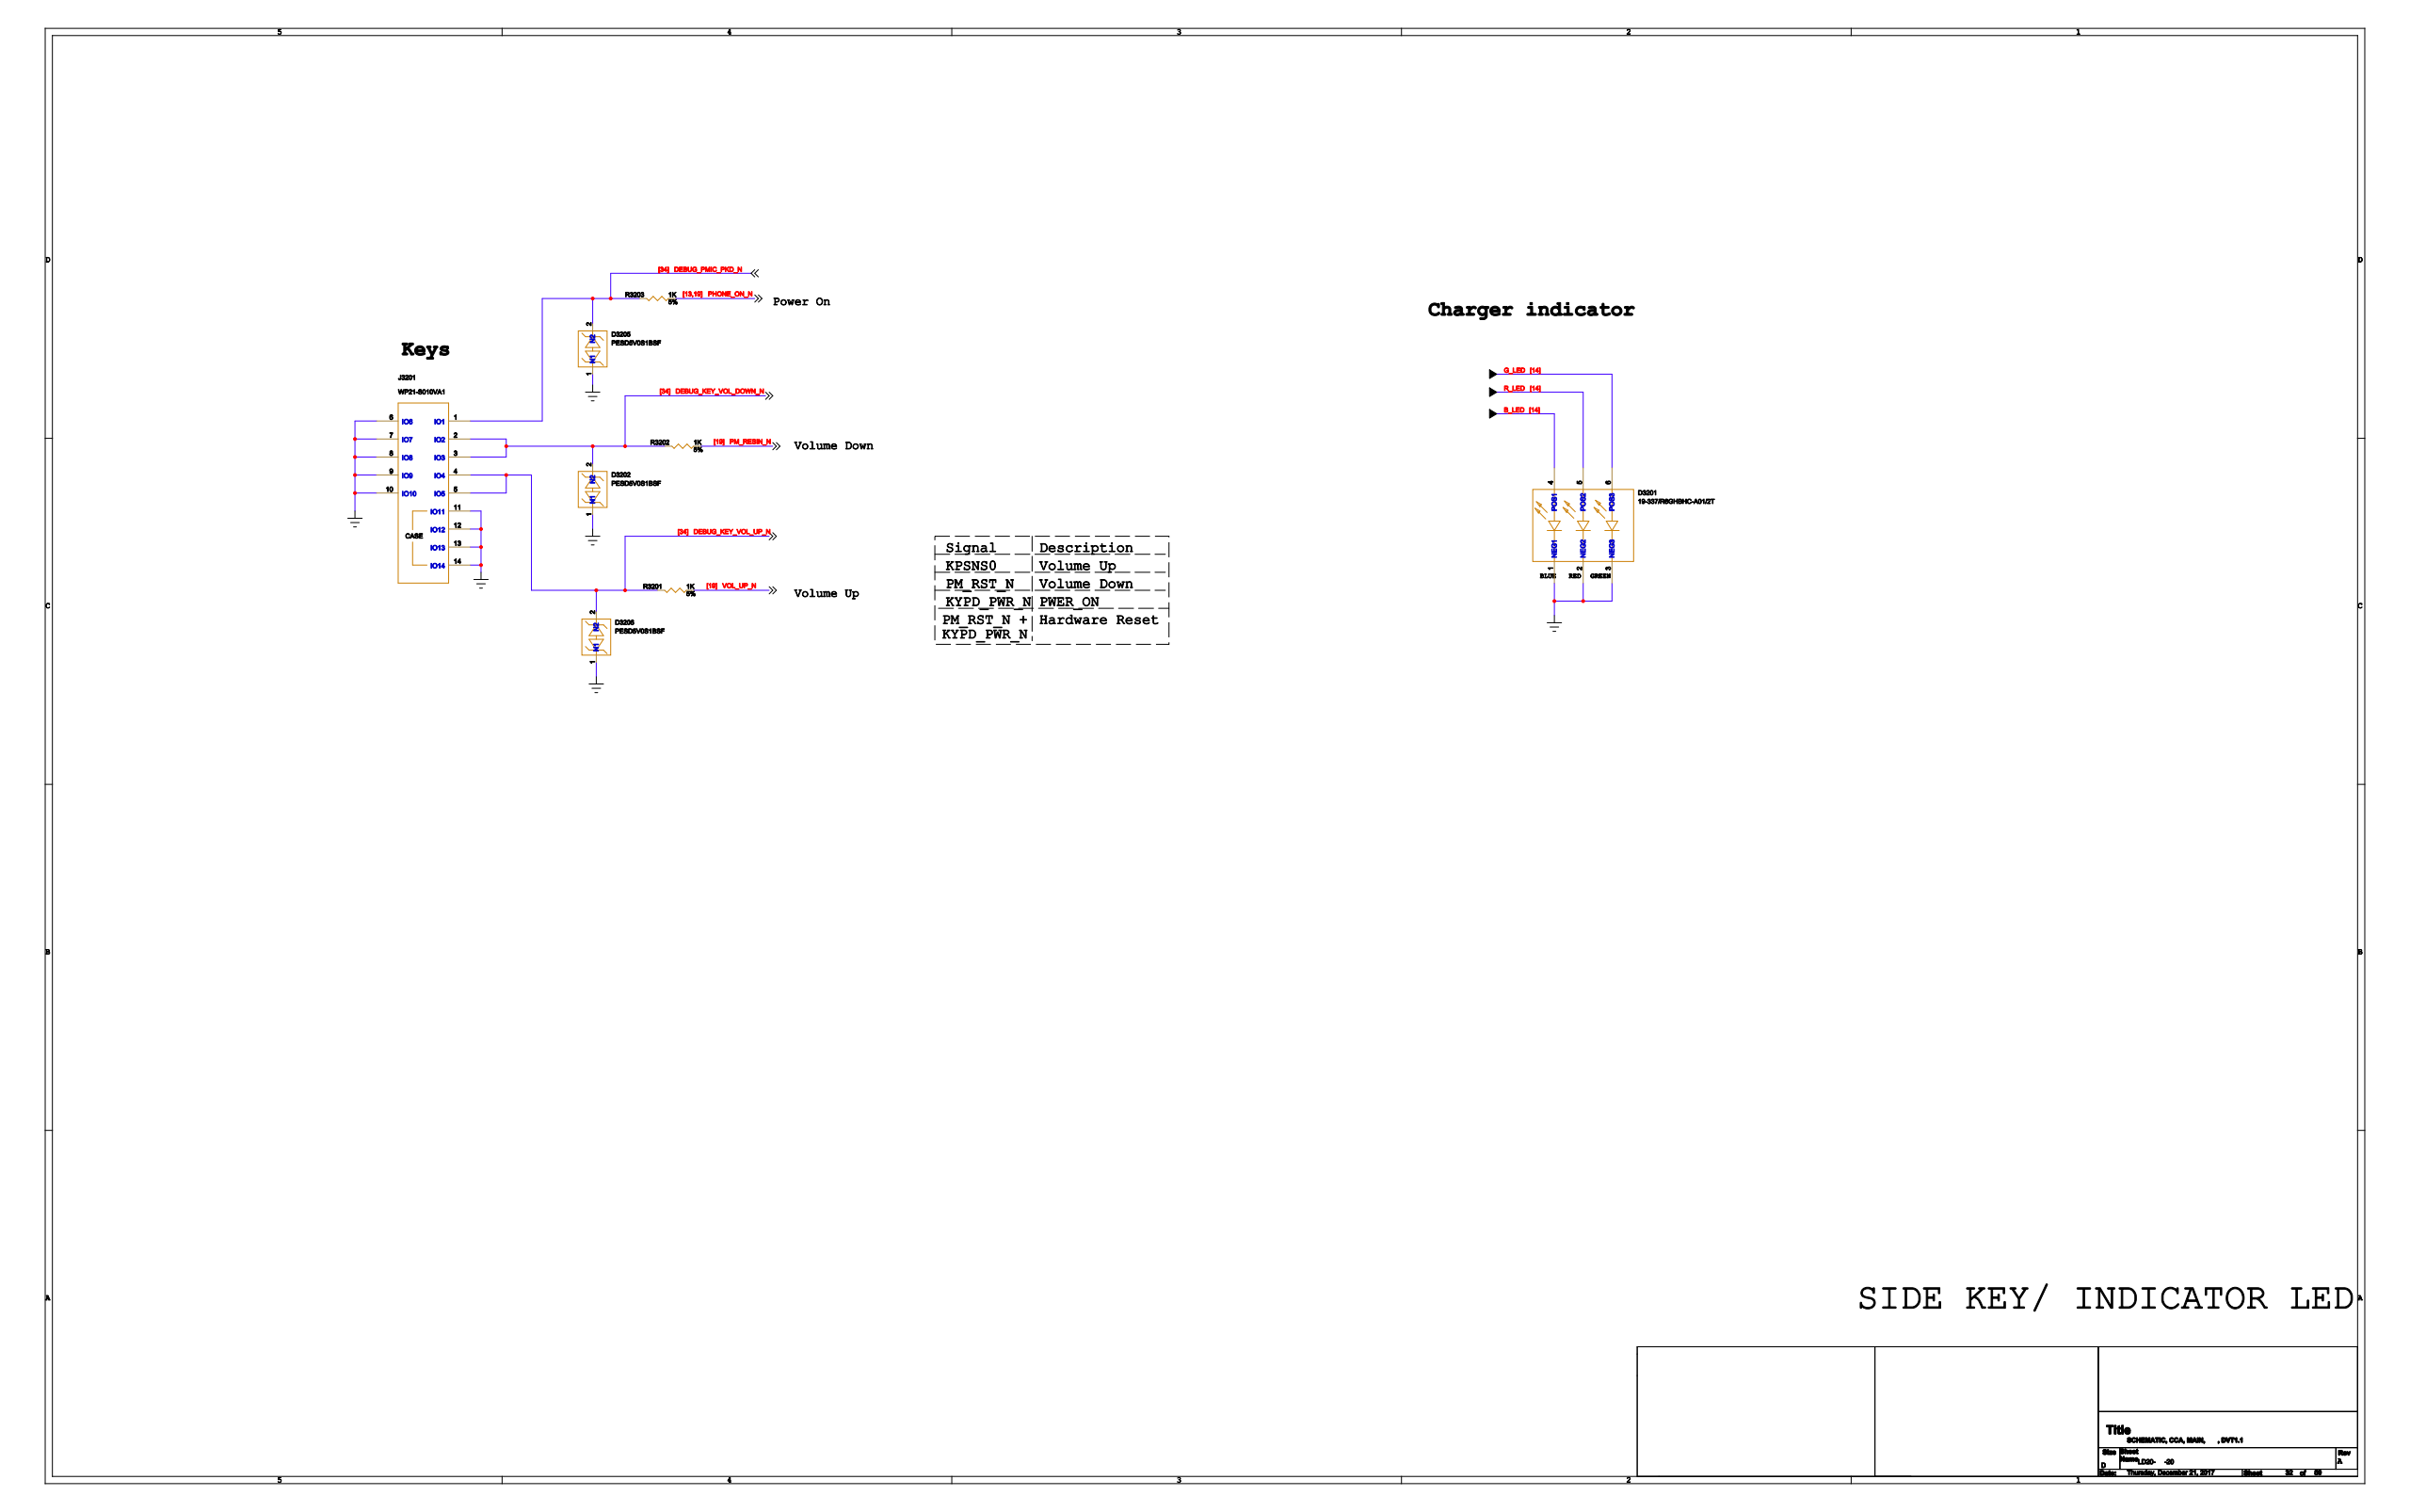Circuit board | Cadence Allegro | 1520 parts | 1149 nets | one sheet of the schematic
Parts on this sheet (reference | value | footprint):
D3201 | 19-337/R6GHBHC-A01/2T | 6PSM67X67N
D3202 | PESD5V0S1BSF | 2PSM25X13N
D3205 | PESD5V0S1BSF | 2PSM25X13N
D3206 | PESD5V0S1BSF | 2PSM25X13N
J3201 | WP21-S010VA1 | 14SCONS138_CCW
R3201 | 1K | 2P0201R
R3202 | 1K | 2P0201R
R3203 | 1K | 2P0201R
Nets of these parts (net: part-pin ...):
GND: D3201-1 D3201-2 D3201-3 D3202-1 D3205-1 D3206-1 J3201-6 J3201-7 J3201-8 J3201-9 J3201-10 J3201-11 J3201-12 J3201-13 J3201-14
DEBUG_KEY_VOL_DOWN_N: D3202-2 J3201-2 J3201-3 R3202-1
DEBUG_PMIC_PKD_N: D3205-2 J3201-1 R3203-1
DEBUG_KEY_VOL_UP_N: D3206-2 J3201-4 J3201-5 R3201-1
B_LED: D3201-4
R_LED: D3201-5
G_LED: D3201-6
VOL_UP_N: R3201-2
PM_RESIN_N: R3202-2
PHONE_ON_N: R3203-2